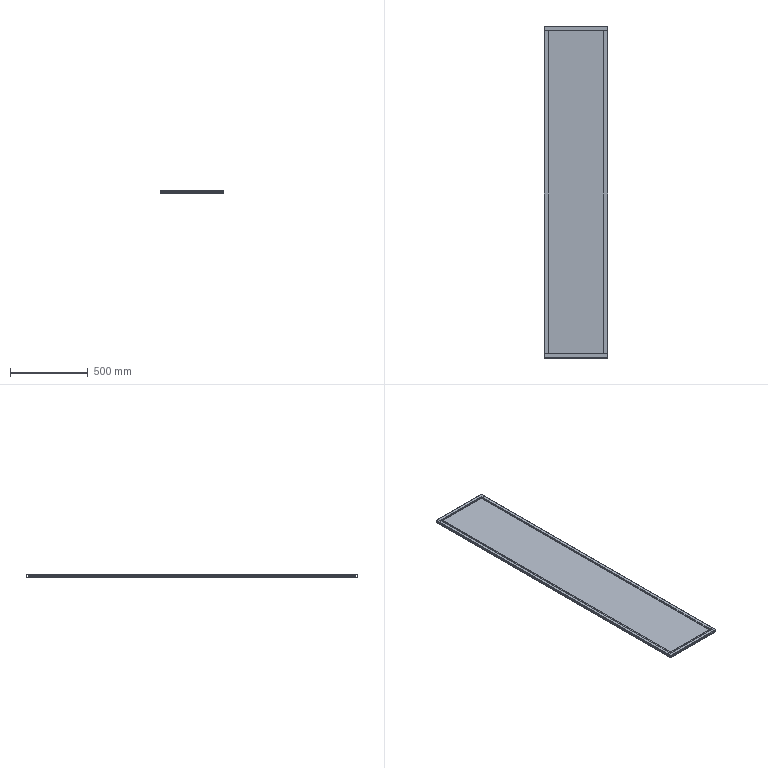Part | SolidWorks | features ICE 2, WeldMemberFeat 1, WeldmentFeature 1 | 5 solids | 167 faces | box 410 x 2136 x 18 mm | volume 8644224 mm3 | plane 98 | cylinder 69 | commonest cylinder face diameters 1.1 x24 3.6 x20 5.8 x20 1 x5